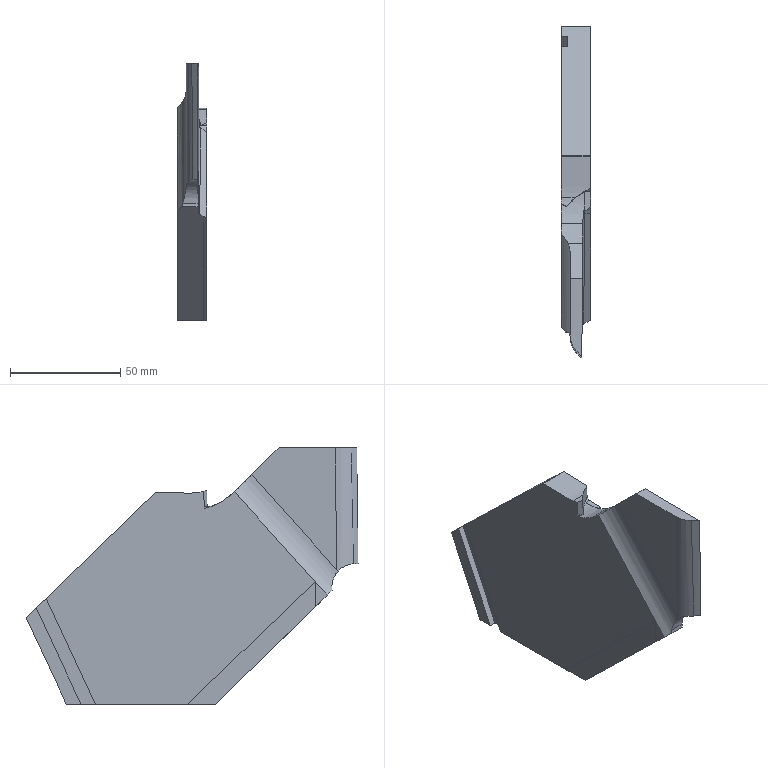Part | Creo | 1 solid | 40 faces | box 13.289 x 150.806 x 116.375 mm | volume 127298 mm3 | plane 23 | cylinder 12 | other 3 | spline 2 | commonest cylinder face diameters 52.26 x2 4.041 x1 21.303 x1 21.31 x1 21.35 x1 22.161 x1